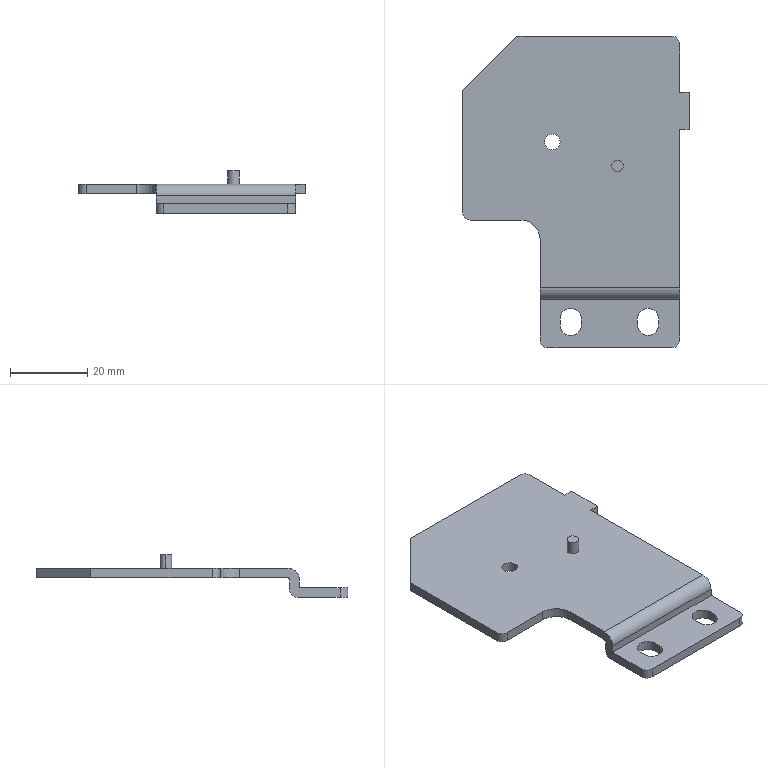Part | NX | features BREP 1 | 1 solid | 38 faces | box 58.5 x 80.5 x 11 mm | volume 9624 mm3 | plane 22 | cylinder 16 | commonest cylinder face diameters 4 x7 5.5 x4 3 x2 1 x1 6 x1 10 x1
STEP:
#1=CARTESIAN_POINT('',(-2.875,12.95,-2.5));
#2=VERTEX_POINT('',#1);
#3=CARTESIAN_POINT('',(-6.875,12.95,-2.5));
#4=VERTEX_POINT('',#3);
#5=CARTESIAN_POINT('',(-4.875,12.95,-2.5));
#6=DIRECTION('',(0.,0.,-1.));
#7=DIRECTION('',(1.,0.,0.));
#8=AXIS2_PLACEMENT_3D('',#5,#6,#7);
#9=CIRCLE('',#8,2.);
#10=EDGE_CURVE('',#2,#4,#9,.T.);
#11=ORIENTED_EDGE('',*,*,#10,.T.);
#12=CARTESIAN_POINT('',(-6.875,12.95,0.));
#13=VERTEX_POINT('',#12);
#14=CARTESIAN_POINT('',(-6.875,12.95,-1.));
#15=DIRECTION('',(0.,0.,1.));
#16=VECTOR('',#15,1000.);
#17=LINE('',#14,#16);
#18=EDGE_CURVE('',#4,#13,#17,.T.);
#19=ORIENTED_EDGE('',*,*,#18,.T.);
#20=CARTESIAN_POINT('',(-2.875,12.95,0.));
#21=VERTEX_POINT('',#20);
#22=CARTESIAN_POINT('',(-4.875,12.95,0.));
#23=DIRECTION('',(0.,0.,-1.));
#24=DIRECTION('',(1.,0.,0.));
#25=AXIS2_PLACEMENT_3D('',#22,#23,#24);
#26=CIRCLE('',#25,2.);
#27=EDGE_CURVE('',#21,#13,#26,.T.);
#28=ORIENTED_EDGE('',*,*,#27,.F.);
#29=CARTESIAN_POINT('',(-2.875,12.95,-1.));
#30=DIRECTION('',(0.,0.,1.));
#31=VECTOR('',#30,1000.);
#32=LINE('',#29,#31);
#33=EDGE_CURVE('',#2,#21,#32,.T.);
#34=ORIENTED_EDGE('',*,*,#33,.F.);
#35=EDGE_LOOP('',(#11,#19,#28,#34));
#36=FACE_BOUND('',#35,.T.);
#37=CARTESIAN_POINT('',(-4.875,12.95,-1.));
#38=DIRECTION('',(0.,0.,1.));
#39=DIRECTION('',(-1.,0.,0.));
#40=AXIS2_PLACEMENT_3D('',#37,#38,#39);
#41=CYLINDRICAL_SURFACE('',#40,2.);
#42=ADVANCED_FACE('',(#36),#41,.F.);
#43=CARTESIAN_POINT('',(10.5,6.75,3.5));
#44=VERTEX_POINT('',#43);
#45=CARTESIAN_POINT('',(13.5,6.75,3.5));
#46=VERTEX_POINT('',#45);
#47=CARTESIAN_POINT('',(12.,6.75,3.5));
#48=DIRECTION('',(0.,0.,-1.));
#49=DIRECTION('',(-1.,0.,0.));
#50=AXIS2_PLACEMENT_3D('',#47,#48,#49);
#51=CIRCLE('',#50,1.5);
#52=EDGE_CURVE('',#44,#46,#51,.T.);
#53=ORIENTED_EDGE('',*,*,#52,.T.);
#54=CARTESIAN_POINT('',(13.5,6.75,0.));
#55=VERTEX_POINT('',#54);
#56=CARTESIAN_POINT('',(13.5,6.75,-2.5));
#57=DIRECTION('',(0.,0.,-1.));
#58=VECTOR('',#57,1000.);
#59=LINE('',#56,#58);
#60=EDGE_CURVE('',#55,#46,#59,.F.);
#61=ORIENTED_EDGE('',*,*,#60,.F.);
#62=CARTESIAN_POINT('',(10.5,6.75,0.));
#63=VERTEX_POINT('',#62);
#64=CARTESIAN_POINT('',(12.,6.75,0.));
#65=DIRECTION('',(0.,0.,-1.));
#66=DIRECTION('',(-1.,0.,0.));
#67=AXIS2_PLACEMENT_3D('',#64,#65,#66);
#68=CIRCLE('',#67,1.5);
#69=EDGE_CURVE('',#63,#55,#68,.T.);
#70=ORIENTED_EDGE('',*,*,#69,.F.);
#71=CARTESIAN_POINT('',(10.5,6.75,-2.5));
#72=DIRECTION('',(0.,0.,-1.));
#73=VECTOR('',#72,1000.);
#74=LINE('',#71,#73);
#75=EDGE_CURVE('',#63,#44,#74,.F.);
#76=ORIENTED_EDGE('',*,*,#75,.T.);
#77=EDGE_LOOP('',(#53,#61,#70,#76));
#78=FACE_BOUND('',#77,.T.);
#79=CARTESIAN_POINT('',(12.,6.75,-2.5));
#80=DIRECTION('',(0.,0.,-1.));
#81=DIRECTION('',(1.,0.,0.));
#82=AXIS2_PLACEMENT_3D('',#79,#80,#81);
#83=CYLINDRICAL_SURFACE('',#82,1.5);
#84=ADVANCED_FACE('',(#78),#83,.T.);
#85=CARTESIAN_POINT('',(-14.,40.25,-2.5));
#86=VERTEX_POINT('',#85);
#87=CARTESIAN_POINT('',(-28.,26.25,-2.5));
#88=VERTEX_POINT('',#87);
#89=CARTESIAN_POINT('',(-14.,40.25,-2.5));
#90=DIRECTION('',(-0.7071,-0.7071,0.));
#91=VECTOR('',#90,1000.);
#92=LINE('',#89,#91);
#93=EDGE_CURVE('',#86,#88,#92,.T.);
#94=ORIENTED_EDGE('',*,*,#93,.F.);
#95=CARTESIAN_POINT('',(26.,40.25,-2.5));
#96=VERTEX_POINT('',#95);
#97=CARTESIAN_POINT('',(38.,40.25,-2.5));
#98=DIRECTION('',(-1.,0.,0.));
#99=VECTOR('',#98,1000.);
#100=LINE('',#97,#99);
#101=EDGE_CURVE('',#96,#86,#100,.T.);
#102=ORIENTED_EDGE('',*,*,#101,.F.);
#103=CARTESIAN_POINT('',(28.,38.25,-2.5));
#104=VERTEX_POINT('',#103);
#105=CARTESIAN_POINT('',(26.,38.25,-2.5));
#106=DIRECTION('',(0.,0.,1.));
#107=DIRECTION('',(1.,0.,0.));
#108=AXIS2_PLACEMENT_3D('',#105,#106,#107);
#109=CIRCLE('',#108,2.);
#110=EDGE_CURVE('',#104,#96,#109,.T.);
#111=ORIENTED_EDGE('',*,*,#110,.F.);
#112=CARTESIAN_POINT('',(28.,25.75,-2.5));
#113=VERTEX_POINT('',#112);
#114=CARTESIAN_POINT('',(28.,-7.834,-2.5));
#115=DIRECTION('',(0.,1.,0.));
#116=VECTOR('',#115,1000.);
#117=LINE('',#114,#116);
#118=EDGE_CURVE('',#113,#104,#117,.T.);
#119=ORIENTED_EDGE('',*,*,#118,.F.);
#120=CARTESIAN_POINT('',(30.5,25.75,-2.5));
#121=VERTEX_POINT('',#120);
#122=CARTESIAN_POINT('',(38.,25.75,-2.5));
#123=DIRECTION('',(-1.,0.,0.));
#124=VECTOR('',#123,1000.);
#125=LINE('',#122,#124);
#126=EDGE_CURVE('',#121,#113,#125,.T.);
#127=ORIENTED_EDGE('',*,*,#126,.F.);
#128=CARTESIAN_POINT('',(30.5,16.25,-2.5));
#129=VERTEX_POINT('',#128);
#130=CARTESIAN_POINT('',(30.5,-7.834,-2.5));
#131=DIRECTION('',(0.,1.,0.));
#132=VECTOR('',#131,1000.);
#133=LINE('',#130,#132);
#134=EDGE_CURVE('',#129,#121,#133,.T.);
#135=ORIENTED_EDGE('',*,*,#134,.F.);
#136=CARTESIAN_POINT('',(28.,16.25,-2.5));
#137=VERTEX_POINT('',#136);
#138=CARTESIAN_POINT('',(38.,16.25,-2.5));
#139=DIRECTION('',(1.,0.,0.));
#140=VECTOR('',#139,1000.);
#141=LINE('',#138,#140);
#142=EDGE_CURVE('',#137,#129,#141,.T.);
#143=ORIENTED_EDGE('',*,*,#142,.F.);
#144=CARTESIAN_POINT('',(28.,-24.768,-2.5));
#145=VERTEX_POINT('',#144);
#146=CARTESIAN_POINT('',(28.,-7.834,-2.5));
#147=DIRECTION('',(0.,1.,0.));
#148=VECTOR('',#147,1000.);
#149=LINE('',#146,#148);
#150=EDGE_CURVE('',#145,#137,#149,.T.);
#151=ORIENTED_EDGE('',*,*,#150,.F.);
#152=CARTESIAN_POINT('',(-8.,-24.768,-2.5));
#153=VERTEX_POINT('',#152);
#154=CARTESIAN_POINT('',(38.,-24.768,-2.5));
#155=DIRECTION('',(1.,0.,0.));
#156=VECTOR('',#155,1000.);
#157=LINE('',#154,#156);
#158=EDGE_CURVE('',#153,#145,#157,.T.);
#159=ORIENTED_EDGE('',*,*,#158,.F.);
#160=CARTESIAN_POINT('',(-8.,-12.25,-2.5));
#161=VERTEX_POINT('',#160);
#162=CARTESIAN_POINT('',(-8.,-7.834,-2.5));
#163=DIRECTION('',(0.,-1.,0.));
#164=VECTOR('',#163,1000.);
#165=LINE('',#162,#164);
#166=EDGE_CURVE('',#161,#153,#165,.T.);
#167=ORIENTED_EDGE('',*,*,#166,.F.);
#168=CARTESIAN_POINT('',(-13.,-7.25,-2.5));
#169=VERTEX_POINT('',#168);
#170=CARTESIAN_POINT('',(-13.,-12.25,-2.5));
#171=DIRECTION('',(0.,0.,-1.));
#172=DIRECTION('',(1.,0.,0.));
#173=AXIS2_PLACEMENT_3D('',#170,#171,#172);
#174=CIRCLE('',#173,5.);
#175=EDGE_CURVE('',#169,#161,#174,.T.);
#176=ORIENTED_EDGE('',*,*,#175,.F.);
#177=CARTESIAN_POINT('',(-26.,-7.25,-2.5));
#178=VERTEX_POINT('',#177);
#179=CARTESIAN_POINT('',(38.,-7.25,-2.5));
#180=DIRECTION('',(1.,0.,0.));
#181=VECTOR('',#180,1000.);
#182=LINE('',#179,#181);
#183=EDGE_CURVE('',#178,#169,#182,.T.);
#184=ORIENTED_EDGE('',*,*,#183,.F.);
#185=CARTESIAN_POINT('',(-28.,-5.25,-2.5));
#186=VERTEX_POINT('',#185);
#187=CARTESIAN_POINT('',(-26.,-5.25,-2.5));
#188=DIRECTION('',(0.,0.,1.));
#189=DIRECTION('',(1.,0.,0.));
#190=AXIS2_PLACEMENT_3D('',#187,#188,#189);
#191=CIRCLE('',#190,2.);
#192=EDGE_CURVE('',#186,#178,#191,.T.);
#193=ORIENTED_EDGE('',*,*,#192,.F.);
#194=CARTESIAN_POINT('',(-28.,-7.834,-2.5));
#195=DIRECTION('',(0.,-1.,0.));
#196=VECTOR('',#195,1000.);
#197=LINE('',#194,#196);
#198=EDGE_CURVE('',#88,#186,#197,.T.);
#199=ORIENTED_EDGE('',*,*,#198,.F.);
#200=EDGE_LOOP('',(#94,#102,#111,#119,#127,#135,#143,#151,#159,#167,#176,#184,#193,#199));
#201=FACE_BOUND('',#200,.T.);
#202=ORIENTED_EDGE('',*,*,#10,.F.);
#203=CARTESIAN_POINT('',(-4.875,12.95,-2.5));
#204=DIRECTION('',(0.,0.,-1.));
#205=DIRECTION('',(1.,0.,0.));
#206=AXIS2_PLACEMENT_3D('',#203,#204,#205);
#207=CIRCLE('',#206,2.);
#208=EDGE_CURVE('',#4,#2,#207,.T.);
#209=ORIENTED_EDGE('',*,*,#208,.F.);
#210=EDGE_LOOP('',(#202,#209));
#211=FACE_BOUND('',#210,.T.);
#212=CARTESIAN_POINT('',(38.,-7.834,-2.5));
#213=DIRECTION('',(0.,0.,1.));
#214=DIRECTION('',(-1.,0.,0.));
#215=AXIS2_PLACEMENT_3D('',#212,#213,#214);
#216=PLANE('',#215);
#217=ADVANCED_FACE('',(#201,#211),#216,.F.);
#218=ORIENTED_EDGE('',*,*,#198,.T.);
#219=CARTESIAN_POINT('',(-28.,-5.25,0.));
#220=VERTEX_POINT('',#219);
#221=CARTESIAN_POINT('',(-28.,-5.25,-1.));
#222=DIRECTION('',(0.,0.,-1.));
#223=VECTOR('',#222,1000.);
#224=LINE('',#221,#223);
#225=EDGE_CURVE('',#220,#186,#224,.T.);
#226=ORIENTED_EDGE('',*,*,#225,.F.);
#227=CARTESIAN_POINT('',(-28.,26.25,0.));
#228=VERTEX_POINT('',#227);
#229=CARTESIAN_POINT('',(-28.,-7.834,0.));
#230=DIRECTION('',(0.,-1.,0.));
#231=VECTOR('',#230,1000.);
#232=LINE('',#229,#231);
#233=EDGE_CURVE('',#228,#220,#232,.T.);
#234=ORIENTED_EDGE('',*,*,#233,.F.);
#235=CARTESIAN_POINT('',(-28.,26.25,-1.));
#236=DIRECTION('',(0.,0.,1.));
#237=VECTOR('',#236,1000.);
#238=LINE('',#235,#237);
#239=EDGE_CURVE('',#88,#228,#238,.T.);
#240=ORIENTED_EDGE('',*,*,#239,.F.);
#241=EDGE_LOOP('',(#218,#226,#234,#240));
#242=FACE_BOUND('',#241,.T.);
#243=CARTESIAN_POINT('',(-28.,-7.834,-1.));
#244=DIRECTION('',(1.,0.,0.));
#245=DIRECTION('',(0.,0.,1.));
#246=AXIS2_PLACEMENT_3D('',#243,#244,#245);
#247=PLANE('',#246);
#248=ADVANCED_FACE('',(#242),#247,.F.);
#249=ORIENTED_EDGE('',*,*,#239,.T.);
#250=CARTESIAN_POINT('',(-14.,40.25,0.));
#251=VERTEX_POINT('',#250);
#252=CARTESIAN_POINT('',(-14.,40.25,0.));
#253=DIRECTION('',(0.7071,0.7071,0.));
#254=VECTOR('',#253,1000.);
#255=LINE('',#252,#254);
#256=EDGE_CURVE('',#228,#251,#255,.T.);
#257=ORIENTED_EDGE('',*,*,#256,.T.);
#258=CARTESIAN_POINT('',(-14.,40.25,-1.));
#259=DIRECTION('',(0.,0.,-1.));
#260=VECTOR('',#259,1000.);
#261=LINE('',#258,#260);
#262=EDGE_CURVE('',#251,#86,#261,.T.);
#263=ORIENTED_EDGE('',*,*,#262,.T.);
#264=ORIENTED_EDGE('',*,*,#93,.T.);
#265=EDGE_LOOP('',(#249,#257,#263,#264));
#266=FACE_BOUND('',#265,.T.);
#267=CARTESIAN_POINT('',(-14.,40.25,-1.));
#268=DIRECTION('',(-0.7071,0.7071,0.));
#269=DIRECTION('',(0.7071,0.7071,0.));
#270=AXIS2_PLACEMENT_3D('',#267,#268,#269);
#271=PLANE('',#270);
#272=ADVANCED_FACE('',(#266),#271,.T.);
#273=ORIENTED_EDGE('',*,*,#101,.T.);
#274=ORIENTED_EDGE('',*,*,#262,.F.);
#275=CARTESIAN_POINT('',(26.,40.25,0.));
#276=VERTEX_POINT('',#275);
#277=CARTESIAN_POINT('',(38.,40.25,0.));
#278=DIRECTION('',(-1.,0.,0.));
#279=VECTOR('',#278,1000.);
#280=LINE('',#277,#279);
#281=EDGE_CURVE('',#276,#251,#280,.T.);
#282=ORIENTED_EDGE('',*,*,#281,.F.);
#283=CARTESIAN_POINT('',(26.,40.25,-1.));
#284=DIRECTION('',(0.,0.,1.));
#285=VECTOR('',#284,1000.);
#286=LINE('',#283,#285);
#287=EDGE_CURVE('',#96,#276,#286,.T.);
#288=ORIENTED_EDGE('',*,*,#287,.F.);
#289=EDGE_LOOP('',(#273,#274,#282,#288));
#290=FACE_BOUND('',#289,.T.);
#291=CARTESIAN_POINT('',(38.,40.25,-1.));
#292=DIRECTION('',(0.,-1.,0.));
#293=DIRECTION('',(0.,0.,1.));
#294=AXIS2_PLACEMENT_3D('',#291,#292,#293);
#295=PLANE('',#294);
#296=ADVANCED_FACE('',(#290),#295,.F.);
#297=ORIENTED_EDGE('',*,*,#287,.T.);
#298=CARTESIAN_POINT('',(28.,38.25,0.));
#299=VERTEX_POINT('',#298);
#300=CARTESIAN_POINT('',(26.,38.25,0.));
#301=DIRECTION('',(0.,0.,-1.));
#302=DIRECTION('',(1.,0.,0.));
#303=AXIS2_PLACEMENT_3D('',#300,#301,#302);
#304=CIRCLE('',#303,2.);
#305=EDGE_CURVE('',#276,#299,#304,.T.);
#306=ORIENTED_EDGE('',*,*,#305,.T.);
#307=CARTESIAN_POINT('',(28.,38.25,-1.));
#308=DIRECTION('',(0.,0.,-1.));
#309=VECTOR('',#308,1000.);
#310=LINE('',#307,#309);
#311=EDGE_CURVE('',#299,#104,#310,.T.);
#312=ORIENTED_EDGE('',*,*,#311,.T.);
#313=ORIENTED_EDGE('',*,*,#110,.T.);
#314=EDGE_LOOP('',(#297,#306,#312,#313));
#315=FACE_BOUND('',#314,.T.);
#316=CARTESIAN_POINT('',(26.,38.25,-1.));
#317=DIRECTION('',(0.,0.,1.));
#318=DIRECTION('',(-1.,0.,0.));
#319=AXIS2_PLACEMENT_3D('',#316,#317,#318);
#320=CYLINDRICAL_SURFACE('',#319,2.);
#321=ADVANCED_FACE('',(#315),#320,.T.);
#322=ORIENTED_EDGE('',*,*,#118,.T.);
#323=ORIENTED_EDGE('',*,*,#311,.F.);
#324=CARTESIAN_POINT('',(28.,25.75,0.));
#325=VERTEX_POINT('',#324);
#326=CARTESIAN_POINT('',(28.,-36.323,0.));
#327=DIRECTION('',(0.,1.,0.));
#328=VECTOR('',#327,1000.);
#329=LINE('',#326,#328);
#330=EDGE_CURVE('',#325,#299,#329,.T.);
#331=ORIENTED_EDGE('',*,*,#330,.F.);
#332=CARTESIAN_POINT('',(28.,25.75,-6.));
#333=DIRECTION('',(0.,0.,1.));
#334=VECTOR('',#333,1000.);
#335=LINE('',#332,#334);
#336=EDGE_CURVE('',#113,#325,#335,.T.);
#337=ORIENTED_EDGE('',*,*,#336,.F.);
#338=EDGE_LOOP('',(#322,#323,#331,#337));
#339=FACE_BOUND('',#338,.T.);
#340=CARTESIAN_POINT('',(28.,-36.323,-6.));
#341=DIRECTION('',(-1.,0.,0.));
#342=DIRECTION('',(0.,0.,-1.));
#343=AXIS2_PLACEMENT_3D('',#340,#341,#342);
#344=PLANE('',#343);
#345=ADVANCED_FACE('',(#339),#344,.F.);
#346=CARTESIAN_POINT('',(30.5,25.75,0.));
#347=VERTEX_POINT('',#346);
#348=CARTESIAN_POINT('',(30.5,25.75,-1.));
#349=DIRECTION('',(0.,0.,1.));
#350=VECTOR('',#349,1000.);
#351=LINE('',#348,#350);
#352=EDGE_CURVE('',#121,#347,#351,.T.);
#353=ORIENTED_EDGE('',*,*,#352,.F.);
#354=ORIENTED_EDGE('',*,*,#126,.T.);
#355=ORIENTED_EDGE('',*,*,#336,.T.);
#356=CARTESIAN_POINT('',(28.,25.75,0.));
#357=DIRECTION('',(-1.,0.,0.));
#358=VECTOR('',#357,1000.);
#359=LINE('',#356,#358);
#360=EDGE_CURVE('',#347,#325,#359,.T.);
#361=ORIENTED_EDGE('',*,*,#360,.F.);
#362=EDGE_LOOP('',(#353,#354,#355,#361));
#363=FACE_BOUND('',#362,.T.);
#364=CARTESIAN_POINT('',(28.,25.75,-1.));
#365=DIRECTION('',(0.,-1.,0.));
#366=DIRECTION('',(0.,0.,1.));
#367=AXIS2_PLACEMENT_3D('',#364,#365,#366);
#368=PLANE('',#367);
#369=ADVANCED_FACE('',(#363),#368,.F.);
#370=ORIENTED_EDGE('',*,*,#134,.T.);
#371=ORIENTED_EDGE('',*,*,#352,.T.);
#372=CARTESIAN_POINT('',(30.5,16.25,0.));
#373=VERTEX_POINT('',#372);
#374=CARTESIAN_POINT('',(30.5,16.25,0.));
#375=DIRECTION('',(0.,1.,0.));
#376=VECTOR('',#375,1000.);
#377=LINE('',#374,#376);
#378=EDGE_CURVE('',#373,#347,#377,.T.);
#379=ORIENTED_EDGE('',*,*,#378,.F.);
#380=CARTESIAN_POINT('',(30.5,16.25,-1.));
#381=DIRECTION('',(0.,0.,1.));
#382=VECTOR('',#381,1000.);
#383=LINE('',#380,#382);
#384=EDGE_CURVE('',#129,#373,#383,.T.);
#385=ORIENTED_EDGE('',*,*,#384,.F.);
#386=EDGE_LOOP('',(#370,#371,#379,#385));
#387=FACE_BOUND('',#386,.T.);
#388=CARTESIAN_POINT('',(30.5,16.25,-1.));
#389=DIRECTION('',(-1.,0.,0.));
#390=DIRECTION('',(0.,0.,-1.));
#391=AXIS2_PLACEMENT_3D('',#388,#389,#390);
#392=PLANE('',#391);
#393=ADVANCED_FACE('',(#387),#392,.F.);
#394=CARTESIAN_POINT('',(28.,16.25,0.));
#395=VERTEX_POINT('',#394);
#396=CARTESIAN_POINT('',(28.,16.25,-1.));
#397=DIRECTION('',(0.,0.,1.));
#398=VECTOR('',#397,1000.);
#399=LINE('',#396,#398);
#400=EDGE_CURVE('',#137,#395,#399,.T.);
#401=ORIENTED_EDGE('',*,*,#400,.F.);
#402=ORIENTED_EDGE('',*,*,#142,.T.);
#403=ORIENTED_EDGE('',*,*,#384,.T.);
#404=CARTESIAN_POINT('',(28.,16.25,0.));
#405=DIRECTION('',(1.,0.,0.));
#406=VECTOR('',#405,1000.);
#407=LINE('',#404,#406);
#408=EDGE_CURVE('',#395,#373,#407,.T.);
#409=ORIENTED_EDGE('',*,*,#408,.F.);
#410=EDGE_LOOP('',(#401,#402,#403,#409));
#411=FACE_BOUND('',#410,.T.);
#412=CARTESIAN_POINT('',(28.,16.25,-1.));
#413=DIRECTION('',(0.,1.,0.));
#414=DIRECTION('',(0.,0.,-1.));
#415=AXIS2_PLACEMENT_3D('',#412,#413,#414);
#416=PLANE('',#415);
#417=ADVANCED_FACE('',(#411),#416,.F.);
#418=CARTESIAN_POINT('',(28.,-27.768,-3.));
#419=VERTEX_POINT('',#418);
#420=CARTESIAN_POINT('',(28.,-24.768,0.));
#421=VERTEX_POINT('',#420);
#422=CARTESIAN_POINT('',(28.,-24.768,-3.));
#423=DIRECTION('',(-1.,0.,0.));
#424=DIRECTION('',(0.,0.,1.));
#425=AXIS2_PLACEMENT_3D('',#422,#423,#424);
#426=CIRCLE('',#425,3.);
#427=EDGE_CURVE('',#419,#421,#426,.T.);
#428=ORIENTED_EDGE('',*,*,#427,.F.);
#429=CARTESIAN_POINT('',(28.,-27.768,-5.));
#430=VERTEX_POINT('',#429);
#431=CARTESIAN_POINT('',(28.,-27.768,-6.));
#432=DIRECTION('',(0.,0.,1.));
#433=VECTOR('',#432,1000.);
#434=LINE('',#431,#433);
#435=EDGE_CURVE('',#430,#419,#434,.T.);
#436=ORIENTED_EDGE('',*,*,#435,.F.);
#437=CARTESIAN_POINT('',(28.,-38.25,-5.));
#438=VERTEX_POINT('',#437);
#439=CARTESIAN_POINT('',(28.,-36.323,-5.));
#440=DIRECTION('',(0.,1.,0.));
#441=VECTOR('',#440,1000.);
#442=LINE('',#439,#441);
#443=EDGE_CURVE('',#438,#430,#442,.T.);
#444=ORIENTED_EDGE('',*,*,#443,.F.);
#445=CARTESIAN_POINT('',(28.,-38.25,-7.5));
#446=VERTEX_POINT('',#445);
#447=CARTESIAN_POINT('',(28.,-38.25,-6.));
#448=DIRECTION('',(0.,0.,1.));
#449=VECTOR('',#448,1000.);
#450=LINE('',#447,#449);
#451=EDGE_CURVE('',#446,#438,#450,.T.);
#452=ORIENTED_EDGE('',*,*,#451,.F.);
#453=CARTESIAN_POINT('',(28.,-27.268,-7.5));
#454=VERTEX_POINT('',#453);
#455=CARTESIAN_POINT('',(28.,-36.323,-7.5));
#456=DIRECTION('',(0.,-1.,0.));
#457=VECTOR('',#456,1000.);
#458=LINE('',#455,#457);
#459=EDGE_CURVE('',#454,#446,#458,.T.);
#460=ORIENTED_EDGE('',*,*,#459,.F.);
#461=CARTESIAN_POINT('',(28.,-25.268,-5.5));
#462=VERTEX_POINT('',#461);
#463=CARTESIAN_POINT('',(28.,-27.268,-5.5));
#464=DIRECTION('',(-1.,0.,0.));
#465=DIRECTION('',(0.,0.,1.));
#466=AXIS2_PLACEMENT_3D('',#463,#464,#465);
#467=CIRCLE('',#466,2.);
#468=EDGE_CURVE('',#462,#454,#467,.T.);
#469=ORIENTED_EDGE('',*,*,#468,.F.);
#470=CARTESIAN_POINT('',(28.,-25.268,-3.));
#471=VERTEX_POINT('',#470);
#472=CARTESIAN_POINT('',(28.,-25.268,-6.));
#473=DIRECTION('',(0.,0.,-1.));
#474=VECTOR('',#473,1000.);
#475=LINE('',#472,#474);
#476=EDGE_CURVE('',#471,#462,#475,.T.);
#477=ORIENTED_EDGE('',*,*,#476,.F.);
#478=CARTESIAN_POINT('',(28.,-24.768,-3.));
#479=DIRECTION('',(1.,0.,0.));
#480=DIRECTION('',(0.,0.,1.));
#481=AXIS2_PLACEMENT_3D('',#478,#479,#480);
#482=CIRCLE('',#481,0.5);
#483=EDGE_CURVE('',#145,#471,#482,.T.);
#484=ORIENTED_EDGE('',*,*,#483,.F.);
#485=ORIENTED_EDGE('',*,*,#150,.T.);
#486=ORIENTED_EDGE('',*,*,#400,.T.);
#487=CARTESIAN_POINT('',(28.,-36.323,0.));
#488=DIRECTION('',(0.,1.,0.));
#489=VECTOR('',#488,1000.);
#490=LINE('',#487,#489);
#491=EDGE_CURVE('',#421,#395,#490,.T.);
#492=ORIENTED_EDGE('',*,*,#491,.F.);
#493=EDGE_LOOP('',(#428,#436,#444,#452,#460,#469,#477,#484,#485,#486,#492));
#494=FACE_BOUND('',#493,.T.);
#495=CARTESIAN_POINT('',(28.,-36.323,-6.));
#496=DIRECTION('',(-1.,0.,0.));
#497=DIRECTION('',(0.,0.,-1.));
#498=AXIS2_PLACEMENT_3D('',#495,#496,#497);
#499=PLANE('',#498);
#500=ADVANCED_FACE('',(#494),#499,.F.);
#501=CARTESIAN_POINT('',(-8.,-25.268,-3.));
#502=VERTEX_POINT('',#501);
#503=CARTESIAN_POINT('',(-8.,-24.768,-3.));
#504=DIRECTION('',(1.,0.,0.));
#505=DIRECTION('',(0.,0.,1.));
#506=AXIS2_PLACEMENT_3D('',#503,#504,#505);
#507=CIRCLE('',#506,0.5);
#508=EDGE_CURVE('',#153,#502,#507,.T.);
#509=ORIENTED_EDGE('',*,*,#508,.F.);
#510=ORIENTED_EDGE('',*,*,#158,.T.);
#511=ORIENTED_EDGE('',*,*,#483,.T.);
#512=CARTESIAN_POINT('',(46.085,-25.268,-3.));
#513=DIRECTION('',(1.,0.,0.));
#514=VECTOR('',#513,1000.);
#515=LINE('',#512,#514);
#516=EDGE_CURVE('',#502,#471,#515,.T.);
#517=ORIENTED_EDGE('',*,*,#516,.F.);
#518=EDGE_LOOP('',(#509,#510,#511,#517));
#519=FACE_BOUND('',#518,.T.);
#520=CARTESIAN_POINT('',(46.085,-24.768,-3.));
#521=DIRECTION('',(-1.,0.,0.));
#522=DIRECTION('',(0.,0.,-1.));
#523=AXIS2_PLACEMENT_3D('',#520,#521,#522);
#524=CYLINDRICAL_SURFACE('',#523,0.5);
#525=ADVANCED_FACE('',(#519),#524,.F.);
#526=CARTESIAN_POINT('',(-8.,-27.768,-3.));
#527=VERTEX_POINT('',#526);
#528=CARTESIAN_POINT('',(-8.,-27.768,-5.));
#529=VERTEX_POINT('',#528);
#530=CARTESIAN_POINT('',(-8.,-27.768,-6.));
#531=DIRECTION('',(0.,0.,-1.));
#532=VECTOR('',#531,1000.);
#533=LINE('',#530,#532);
#534=EDGE_CURVE('',#527,#529,#533,.T.);
#535=ORIENTED_EDGE('',*,*,#534,.F.);
#536=CARTESIAN_POINT('',(-8.,-24.768,0.));
#537=VERTEX_POINT('',#536);
#538=CARTESIAN_POINT('',(-8.,-24.768,-3.));
#539=DIRECTION('',(1.,0.,0.));
#540=DIRECTION('',(0.,0.,1.));
#541=AXIS2_PLACEMENT_3D('',#538,#539,#540);
#542=CIRCLE('',#541,3.);
#543=EDGE_CURVE('',#537,#527,#542,.T.);
#544=ORIENTED_EDGE('',*,*,#543,.F.);
#545=CARTESIAN_POINT('',(-8.,-12.25,0.));
#546=VERTEX_POINT('',#545);
#547=CARTESIAN_POINT('',(-8.,32.708,0.));
#548=DIRECTION('',(0.,-1.,0.));
#549=VECTOR('',#548,1000.);
#550=LINE('',#547,#549);
#551=EDGE_CURVE('',#546,#537,#550,.T.);
#552=ORIENTED_EDGE('',*,*,#551,.F.);
#553=CARTESIAN_POINT('',(-8.,-12.25,-6.));
#554=DIRECTION('',(0.,0.,1.));
#555=VECTOR('',#554,1000.);
#556=LINE('',#553,#555);
#557=EDGE_CURVE('',#161,#546,#556,.T.);
#558=ORIENTED_EDGE('',*,*,#557,.F.);
#559=ORIENTED_EDGE('',*,*,#166,.T.);
#560=ORIENTED_EDGE('',*,*,#508,.T.);
#561=CARTESIAN_POINT('',(-8.,-25.268,-5.5));
#562=VERTEX_POINT('',#561);
#563=CARTESIAN_POINT('',(-8.,-25.268,-6.));
#564=DIRECTION('',(0.,0.,1.));
#565=VECTOR('',#564,1000.);
#566=LINE('',#563,#565);
#567=EDGE_CURVE('',#562,#502,#566,.T.);
#568=ORIENTED_EDGE('',*,*,#567,.F.);
#569=CARTESIAN_POINT('',(-8.,-27.268,-7.5));
#570=VERTEX_POINT('',#569);
#571=CARTESIAN_POINT('',(-8.,-27.268,-5.5));
#572=DIRECTION('',(1.,0.,0.));
#573=DIRECTION('',(0.,0.,1.));
#574=AXIS2_PLACEMENT_3D('',#571,#572,#573);
#575=CIRCLE('',#574,2.);
#576=EDGE_CURVE('',#570,#562,#575,.T.);
#577=ORIENTED_EDGE('',*,*,#576,.F.);
#578=CARTESIAN_POINT('',(-8.,-38.25,-7.5));
#579=VERTEX_POINT('',#578);
#580=CARTESIAN_POINT('',(-8.,32.708,-7.5));
#581=DIRECTION('',(0.,1.,0.));
#582=VECTOR('',#581,1000.);
#583=LINE('',#580,#582);
#584=EDGE_CURVE('',#579,#570,#583,.T.);
#585=ORIENTED_EDGE('',*,*,#584,.F.);
#586=CARTESIAN_POINT('',(-8.,-38.25,-5.));
#587=VERTEX_POINT('',#586);
#588=CARTESIAN_POINT('',(-8.,-38.25,-6.));
#589=DIRECTION('',(0.,0.,-1.));
#590=VECTOR('',#589,1000.);
#591=LINE('',#588,#590);
#592=EDGE_CURVE('',#587,#579,#591,.T.);
#593=ORIENTED_EDGE('',*,*,#592,.F.);
#594=CARTESIAN_POINT('',(-8.,32.708,-5.));
#595=DIRECTION('',(0.,-1.,0.));
#596=VECTOR('',#595,1000.);
#597=LINE('',#594,#596);
#598=EDGE_CURVE('',#529,#587,#597,.T.);
#599=ORIENTED_EDGE('',*,*,#598,.F.);
#600=EDGE_LOOP('',(#535,#544,#552,#558,#559,#560,#568,#577,#585,#593,#599));
#601=FACE_BOUND('',#600,.T.);
#602=CARTESIAN_POINT('',(-8.,32.708,-6.));
#603=DIRECTION('',(1.,0.,0.));
#604=DIRECTION('',(0.,0.,1.));
#605=AXIS2_PLACEMENT_3D('',#602,#603,#604);
#606=PLANE('',#605);
#607=ADVANCED_FACE('',(#601),#606,.F.);
#608=CARTESIAN_POINT('',(-13.,-7.25,0.));
#609=VERTEX_POINT('',#608);
#610=CARTESIAN_POINT('',(-13.,-12.25,0.));
#611=DIRECTION('',(0.,0.,-1.));
#612=DIRECTION('',(1.,0.,0.));
#613=AXIS2_PLACEMENT_3D('',#610,#611,#612);
#614=CIRCLE('',#613,5.);
#615=EDGE_CURVE('',#609,#546,#614,.T.);
#616=ORIENTED_EDGE('',*,*,#615,.F.);
#617=CARTESIAN_POINT('',(-13.,-7.25,-1.));
#618=DIRECTION('',(0.,0.,1.));
#619=VECTOR('',#618,1000.);
#620=LINE('',#617,#619);
#621=EDGE_CURVE('',#169,#609,#620,.T.);
#622=ORIENTED_EDGE('',*,*,#621,.F.);
#623=ORIENTED_EDGE('',*,*,#175,.T.);
#624=ORIENTED_EDGE('',*,*,#557,.T.);
#625=EDGE_LOOP('',(#616,#622,#623,#624));
#626=FACE_BOUND('',#625,.T.);
#627=CARTESIAN_POINT('',(-13.,-12.25,-1.));
#628=DIRECTION('',(0.,0.,1.));
#629=DIRECTION('',(-1.,0.,0.));
#630=AXIS2_PLACEMENT_3D('',#627,#628,#629);
#631=CYLINDRICAL_SURFACE('',#630,5.);
#632=ADVANCED_FACE('',(#626),#631,.F.);
#633=ORIENTED_EDGE('',*,*,#621,.T.);
#634=CARTESIAN_POINT('',(-26.,-7.25,0.));
#635=VERTEX_POINT('',#634);
#636=CARTESIAN_POINT('',(38.,-7.25,0.));
#637=DIRECTION('',(-1.,0.,0.));
#638=VECTOR('',#637,1000.);
#639=LINE('',#636,#638);
#640=EDGE_CURVE('',#609,#635,#639,.T.);
#641=ORIENTED_EDGE('',*,*,#640,.T.);
#642=CARTESIAN_POINT('',(-26.,-7.25,-1.));
#643=DIRECTION('',(0.,0.,-1.));
#644=VECTOR('',#643,1000.);
#645=LINE('',#642,#644);
#646=EDGE_CURVE('',#635,#178,#645,.T.);
#647=ORIENTED_EDGE('',*,*,#646,.T.);
#648=ORIENTED_EDGE('',*,*,#183,.T.);
#649=EDGE_LOOP('',(#633,#641,#647,#648));
#650=FACE_BOUND('',#649,.T.);
#651=CARTESIAN_POINT('',(38.,-7.25,-1.));
#652=DIRECTION('',(0.,-1.,0.));
#653=DIRECTION('',(0.,0.,1.));
#654=AXIS2_PLACEMENT_3D('',#651,#652,#653);
#655=PLANE('',#654);
#656=ADVANCED_FACE('',(#650),#655,.T.);
#657=ORIENTED_EDGE('',*,*,#646,.F.);
#658=CARTESIAN_POINT('',(-26.,-5.25,0.));
#659=DIRECTION('',(0.,0.,-1.));
#660=DIRECTION('',(1.,0.,0.));
#661=AXIS2_PLACEMENT_3D('',#658,#659,#660);
#662=CIRCLE('',#661,2.);
#663=EDGE_CURVE('',#635,#220,#662,.T.);
#664=ORIENTED_EDGE('',*,*,#663,.T.);
#665=ORIENTED_EDGE('',*,*,#225,.T.);
#666=ORIENTED_EDGE('',*,*,#192,.T.);
#667=EDGE_LOOP('',(#657,#664,#665,#666));
#668=FACE_BOUND('',#667,.T.);
#669=CARTESIAN_POINT('',(-26.,-5.25,-1.));
#670=DIRECTION('',(0.,0.,1.));
#671=DIRECTION('',(-1.,0.,0.));
#672=AXIS2_PLACEMENT_3D('',#669,#670,#671);
#673=CYLINDRICAL_SURFACE('',#672,2.);
#674=ADVANCED_FACE('',(#668),#673,.T.);
#675=ORIENTED_EDGE('',*,*,#18,.F.);
#676=ORIENTED_EDGE('',*,*,#208,.T.);
#677=ORIENTED_EDGE('',*,*,#33,.T.);
#678=CARTESIAN_POINT('',(-4.875,12.95,0.));
#679=DIRECTION('',(0.,0.,-1.));
#680=DIRECTION('',(1.,0.,0.));
#681=AXIS2_PLACEMENT_3D('',#678,#679,#680);
#682=CIRCLE('',#681,2.);
#683=EDGE_CURVE('',#13,#21,#682,.T.);
#684=ORIENTED_EDGE('',*,*,#683,.F.);
#685=EDGE_LOOP('',(#675,#676,#677,#684));
#686=FACE_BOUND('',#685,.T.);
#687=CARTESIAN_POINT('',(-4.875,12.95,-1.));
#688=DIRECTION('',(0.,0.,1.));
#689=DIRECTION('',(-1.,0.,0.));
#690=AXIS2_PLACEMENT_3D('',#687,#688,#689);
#691=CYLINDRICAL_SURFACE('',#690,2.);
#692=ADVANCED_FACE('',(#686),#691,.F.);
#693=ORIENTED_EDGE('',*,*,#360,.T.);
#694=ORIENTED_EDGE('',*,*,#330,.T.);
#695=ORIENTED_EDGE('',*,*,#305,.F.);
#696=ORIENTED_EDGE('',*,*,#281,.T.);
#697=ORIENTED_EDGE('',*,*,#256,.F.);
#698=ORIENTED_EDGE('',*,*,#233,.T.);
#699=ORIENTED_EDGE('',*,*,#663,.F.);
#700=ORIENTED_EDGE('',*,*,#640,.F.);
#701=ORIENTED_EDGE('',*,*,#615,.T.);
#702=ORIENTED_EDGE('',*,*,#551,.T.);
#703=CARTESIAN_POINT('',(38.,-24.768,0.));
#704=DIRECTION('',(1.,0.,0.));
#705=VECTOR('',#704,1000.);
#706=LINE('',#703,#705);
#707=EDGE_CURVE('',#537,#421,#706,.T.);
#708=ORIENTED_EDGE('',*,*,#707,.T.);
#709=ORIENTED_EDGE('',*,*,#491,.T.);
#710=ORIENTED_EDGE('',*,*,#408,.T.);
#711=ORIENTED_EDGE('',*,*,#378,.T.);
#712=EDGE_LOOP('',(#693,#694,#695,#696,#697,#698,#699,#700,#701,#702,#708,#709,#710,#711));
#713=FACE_BOUND('',#712,.T.);
#714=ORIENTED_EDGE('',*,*,#27,.T.);
#715=ORIENTED_EDGE('',*,*,#683,.T.);
#716=EDGE_LOOP('',(#714,#715));
#717=FACE_BOUND('',#716,.T.);
#718=ORIENTED_EDGE('',*,*,#69,.T.);
#719=CARTESIAN_POINT('',(12.,6.75,0.));
#720=DIRECTION('',(0.,0.,-1.));
#721=DIRECTION('',(-1.,0.,0.));
#722=AXIS2_PLACEMENT_3D('',#719,#720,#721);
#723=CIRCLE('',#722,1.5);
#724=EDGE_CURVE('',#55,#63,#723,.T.);
#725=ORIENTED_EDGE('',*,*,#724,.T.);
#726=EDGE_LOOP('',(#718,#725));
#727=FACE_BOUND('',#726,.T.);
#728=CARTESIAN_POINT('',(38.,-7.834,0.));
#729=DIRECTION('',(0.,0.,1.));
#730=DIRECTION('',(-1.,0.,0.));
#731=AXIS2_PLACEMENT_3D('',#728,#729,#730);
#732=PLANE('',#731);
#733=ADVANCED_FACE('',(#713,#717,#727),#732,.T.);
#734=ORIENTED_EDGE('',*,*,#707,.F.);
#735=ORIENTED_EDGE('',*,*,#543,.T.);
#736=CARTESIAN_POINT('',(46.085,-27.768,-3.));
#737=DIRECTION('',(1.,0.,0.));
#738=VECTOR('',#737,1000.);
#739=LINE('',#736,#738);
#740=EDGE_CURVE('',#527,#419,#739,.T.);
#741=ORIENTED_EDGE('',*,*,#740,.T.);
#742=ORIENTED_EDGE('',*,*,#427,.T.);
#743=EDGE_LOOP('',(#734,#735,#741,#742));
#744=FACE_BOUND('',#743,.T.);
#745=CARTESIAN_POINT('',(46.085,-24.768,-3.));
#746=DIRECTION('',(-1.,0.,0.));
#747=DIRECTION('',(0.,0.,-1.));
#748=AXIS2_PLACEMENT_3D('',#745,#746,#747);
#749=CYLINDRICAL_SURFACE('',#748,3.);
#750=ADVANCED_FACE('',(#744),#749,.T.);
#751=ORIENTED_EDGE('',*,*,#740,.F.);
#752=ORIENTED_EDGE('',*,*,#534,.T.);
#753=CARTESIAN_POINT('',(38.,-27.768,-5.));
#754=DIRECTION('',(1.,0.,0.));
#755=VECTOR('',#754,1000.);
#756=LINE('',#753,#755);
#757=EDGE_CURVE('',#529,#430,#756,.T.);
#758=ORIENTED_EDGE('',*,*,#757,.T.);
#759=ORIENTED_EDGE('',*,*,#435,.T.);
#760=EDGE_LOOP('',(#751,#752,#758,#759));
#761=FACE_BOUND('',#760,.T.);
#762=CARTESIAN_POINT('',(38.,-27.768,15.898));
#763=DIRECTION('',(0.,-1.,0.));
#764=DIRECTION('',(0.,0.,1.));
#765=AXIS2_PLACEMENT_3D('',#762,#763,#764);
#766=PLANE('',#765);
#767=ADVANCED_FACE('',(#761),#766,.T.);
#768=ORIENTED_EDGE('',*,*,#757,.F.);
#769=ORIENTED_EDGE('',*,*,#598,.T.);
#770=CARTESIAN_POINT('',(-6.,-40.25,-5.));
#771=VERTEX_POINT('',#770);
#772=CARTESIAN_POINT('',(-6.,-38.25,-5.));
#773=DIRECTION('',(0.,0.,1.));
#774=DIRECTION('',(1.,0.,0.));
#775=AXIS2_PLACEMENT_3D('',#772,#773,#774);
#776=CIRCLE('',#775,2.);
#777=EDGE_CURVE('',#587,#771,#776,.T.);
#778=ORIENTED_EDGE('',*,*,#777,.T.);
#779=CARTESIAN_POINT('',(26.,-40.25,-5.));
#780=VERTEX_POINT('',#779);
#781=CARTESIAN_POINT('',(38.,-40.25,-5.));
#782=DIRECTION('',(1.,0.,0.));
#783=VECTOR('',#782,1000.);
#784=LINE('',#781,#783);
#785=EDGE_CURVE('',#771,#780,#784,.T.);
#786=ORIENTED_EDGE('',*,*,#785,.T.);
#787=CARTESIAN_POINT('',(26.,-38.25,-5.));
#788=DIRECTION('',(0.,0.,1.));
#789=DIRECTION('',(1.,0.,0.));
#790=AXIS2_PLACEMENT_3D('',#787,#788,#789);
#791=CIRCLE('',#790,2.);
#792=EDGE_CURVE('',#780,#438,#791,.T.);
#793=ORIENTED_EDGE('',*,*,#792,.T.);
#794=ORIENTED_EDGE('',*,*,#443,.T.);
#795=EDGE_LOOP('',(#768,#769,#778,#786,#793,#794));
#796=FACE_BOUND('',#795,.T.);
#797=CARTESIAN_POINT('',(17.125,-32.8,-5.));
#798=VERTEX_POINT('',#797);
#799=CARTESIAN_POINT('',(17.125,-34.3,-5.));
#800=VERTEX_POINT('',#799);
#801=CARTESIAN_POINT('',(17.125,-34.3,-5.));
#802=DIRECTION('',(0.,-1.,0.));
#803=VECTOR('',#802,1000.);
#804=LINE('',#801,#803);
#805=EDGE_CURVE('',#798,#800,#804,.T.);
#806=ORIENTED_EDGE('',*,*,#805,.F.);
#807=CARTESIAN_POINT('',(22.625,-32.8,-5.));
#808=VERTEX_POINT('',#807);
#809=CARTESIAN_POINT('',(19.875,-32.8,-5.));
#810=DIRECTION('',(0.,0.,-1.));
#811=DIRECTION('',(1.,0.,0.));
#812=AXIS2_PLACEMENT_3D('',#809,#810,#811);
#813=CIRCLE('',#812,2.75);
#814=EDGE_CURVE('',#798,#808,#813,.T.);
#815=ORIENTED_EDGE('',*,*,#814,.T.);
#816=CARTESIAN_POINT('',(22.625,-34.3,-5.));
#817=VERTEX_POINT('',#816);
#818=CARTESIAN_POINT('',(22.625,-34.3,-5.));
#819=DIRECTION('',(0.,1.,0.));
#820=VECTOR('',#819,1000.);
#821=LINE('',#818,#820);
#822=EDGE_CURVE('',#817,#808,#821,.T.);
#823=ORIENTED_EDGE('',*,*,#822,.F.);
#824=CARTESIAN_POINT('',(19.875,-34.3,-5.));
#825=DIRECTION('',(0.,0.,-1.));
#826=DIRECTION('',(1.,0.,0.));
#827=AXIS2_PLACEMENT_3D('',#824,#825,#826);
#828=CIRCLE('',#827,2.75);
#829=EDGE_CURVE('',#817,#800,#828,.T.);
#830=ORIENTED_EDGE('',*,*,#829,.T.);
#831=EDGE_LOOP('',(#806,#815,#823,#830));
#832=FACE_BOUND('',#831,.T.);
#833=CARTESIAN_POINT('',(-2.875,-32.8,-5.));
#834=VERTEX_POINT('',#833);
#835=CARTESIAN_POINT('',(-2.875,-34.3,-5.));
#836=VERTEX_POINT('',#835);
#837=CARTESIAN_POINT('',(-2.875,-34.3,-5.));
#838=DIRECTION('',(0.,-1.,0.));
#839=VECTOR('',#838,1000.);
#840=LINE('',#837,#839);
#841=EDGE_CURVE('',#834,#836,#840,.T.);
#842=ORIENTED_EDGE('',*,*,#841,.F.);
#843=CARTESIAN_POINT('',(2.625,-32.8,-5.));
#844=VERTEX_POINT('',#843);
#845=CARTESIAN_POINT('',(-0.125,-32.8,-5.));
#846=DIRECTION('',(0.,0.,-1.));
#847=DIRECTION('',(1.,0.,0.));
#848=AXIS2_PLACEMENT_3D('',#845,#846,#847);
#849=CIRCLE('',#848,2.75);
#850=EDGE_CURVE('',#834,#844,#849,.T.);
#851=ORIENTED_EDGE('',*,*,#850,.T.);
#852=CARTESIAN_POINT('',(2.625,-34.3,-5.));
#853=VERTEX_POINT('',#852);
#854=CARTESIAN_POINT('',(2.625,-34.3,-5.));
#855=DIRECTION('',(0.,1.,0.));
#856=VECTOR('',#855,1000.);
#857=LINE('',#854,#856);
#858=EDGE_CURVE('',#853,#844,#857,.T.);
#859=ORIENTED_EDGE('',*,*,#858,.F.);
#860=CARTESIAN_POINT('',(-0.125,-34.3,-5.));
#861=DIRECTION('',(0.,0.,-1.));
#862=DIRECTION('',(1.,0.,0.));
#863=AXIS2_PLACEMENT_3D('',#860,#861,#862);
#864=CIRCLE('',#863,2.75);
#865=EDGE_CURVE('',#853,#836,#864,.T.);
#866=ORIENTED_EDGE('',*,*,#865,.T.);
#867=EDGE_LOOP('',(#842,#851,#859,#866));
#868=FACE_BOUND('',#867,.T.);
#869=CARTESIAN_POINT('',(38.,-3.907,-5.));
#870=DIRECTION('',(0.,0.,1.));
#871=DIRECTION('',(-1.,0.,0.));
#872=AXIS2_PLACEMENT_3D('',#869,#870,#871);
#873=PLANE('',#872);
#874=ADVANCED_FACE('',(#796,#832,#868),#873,.T.);
#875=ORIENTED_EDGE('',*,*,#451,.T.);
#876=ORIENTED_EDGE('',*,*,#792,.F.);
#877=CARTESIAN_POINT('',(26.,-40.25,-7.5));
#878=VERTEX_POINT('',#877);
#879=CARTESIAN_POINT('',(26.,-40.25,-6.));
#880=DIRECTION('',(0.,0.,-1.));
#881=VECTOR('',#880,1000.);
#882=LINE('',#879,#881);
#883=EDGE_CURVE('',#780,#878,#882,.T.);
#884=ORIENTED_EDGE('',*,*,#883,.T.);
#885=CARTESIAN_POINT('',(26.,-38.25,-7.5));
#886=DIRECTION('',(0.,0.,1.));
#887=DIRECTION('',(1.,0.,0.));
#888=AXIS2_PLACEMENT_3D('',#885,#886,#887);
#889=CIRCLE('',#888,2.);
#890=EDGE_CURVE('',#878,#446,#889,.T.);
#891=ORIENTED_EDGE('',*,*,#890,.T.);
#892=EDGE_LOOP('',(#875,#876,#884,#891));
#893=FACE_BOUND('',#892,.T.);
#894=CARTESIAN_POINT('',(26.,-38.25,-6.));
#895=DIRECTION('',(0.,0.,1.));
#896=DIRECTION('',(-1.,0.,0.));
#897=AXIS2_PLACEMENT_3D('',#894,#895,#896);
#898=CYLINDRICAL_SURFACE('',#897,2.);
#899=ADVANCED_FACE('',(#893),#898,.T.);
#900=ORIENTED_EDGE('',*,*,#584,.T.);
#901=CARTESIAN_POINT('',(38.,-27.268,-7.5));
#902=DIRECTION('',(-1.,0.,0.));
#903=VECTOR('',#902,1000.);
#904=LINE('',#901,#903);
#905=EDGE_CURVE('',#454,#570,#904,.T.);
#906=ORIENTED_EDGE('',*,*,#905,.F.);
#907=ORIENTED_EDGE('',*,*,#459,.T.);
#908=ORIENTED_EDGE('',*,*,#890,.F.);
#909=CARTESIAN_POINT('',(-6.,-40.25,-7.5));
#910=VERTEX_POINT('',#909);
#911=CARTESIAN_POINT('',(38.,-40.25,-7.5));
#912=DIRECTION('',(1.,0.,0.));
#913=VECTOR('',#912,1000.);
#914=LINE('',#911,#913);
#915=EDGE_CURVE('',#910,#878,#914,.T.);
#916=ORIENTED_EDGE('',*,*,#915,.F.);
#917=CARTESIAN_POINT('',(-6.,-38.25,-7.5));
#918=DIRECTION('',(0.,0.,1.));
#919=DIRECTION('',(1.,0.,0.));
#920=AXIS2_PLACEMENT_3D('',#917,#918,#919);
#921=CIRCLE('',#920,2.);
#922=EDGE_CURVE('',#579,#910,#921,.T.);
#923=ORIENTED_EDGE('',*,*,#922,.F.);
#924=EDGE_LOOP('',(#900,#906,#907,#908,#916,#923));
#925=FACE_BOUND('',#924,.T.);
#926=CARTESIAN_POINT('',(17.125,-34.3,-7.5));
#927=VERTEX_POINT('',#926);
#928=CARTESIAN_POINT('',(17.125,-32.8,-7.5));
#929=VERTEX_POINT('',#928);
#930=CARTESIAN_POINT('',(17.125,-34.3,-7.5));
#931=DIRECTION('',(0.,1.,0.));
#932=VECTOR('',#931,1000.);
#933=LINE('',#930,#932);
#934=EDGE_CURVE('',#927,#929,#933,.T.);
#935=ORIENTED_EDGE('',*,*,#934,.F.);
#936=CARTESIAN_POINT('',(22.625,-34.3,-7.5));
#937=VERTEX_POINT('',#936);
#938=CARTESIAN_POINT('',(19.875,-34.3,-7.5));
#939=DIRECTION('',(0.,0.,-1.));
#940=DIRECTION('',(1.,0.,0.));
#941=AXIS2_PLACEMENT_3D('',#938,#939,#940);
#942=CIRCLE('',#941,2.75);
#943=EDGE_CURVE('',#937,#927,#942,.T.);
#944=ORIENTED_EDGE('',*,*,#943,.F.);
#945=CARTESIAN_POINT('',(22.625,-32.8,-7.5));
#946=VERTEX_POINT('',#945);
#947=CARTESIAN_POINT('',(22.625,-34.3,-7.5));
#948=DIRECTION('',(0.,-1.,0.));
#949=VECTOR('',#948,1000.);
#950=LINE('',#947,#949);
#951=EDGE_CURVE('',#946,#937,#950,.T.);
#952=ORIENTED_EDGE('',*,*,#951,.F.);
#953=CARTESIAN_POINT('',(19.875,-32.8,-7.5));
#954=DIRECTION('',(0.,0.,-1.));
#955=DIRECTION('',(1.,0.,0.));
#956=AXIS2_PLACEMENT_3D('',#953,#954,#955);
#957=CIRCLE('',#956,2.75);
#958=EDGE_CURVE('',#929,#946,#957,.T.);
#959=ORIENTED_EDGE('',*,*,#958,.F.);
#960=EDGE_LOOP('',(#935,#944,#952,#959));
#961=FACE_BOUND('',#960,.T.);
#962=CARTESIAN_POINT('',(-2.875,-34.3,-7.5));
#963=VERTEX_POINT('',#962);
#964=CARTESIAN_POINT('',(-2.875,-32.8,-7.5));
#965=VERTEX_POINT('',#964);
#966=CARTESIAN_POINT('',(-2.875,-34.3,-7.5));
#967=DIRECTION('',(0.,1.,0.));
#968=VECTOR('',#967,1000.);
#969=LINE('',#966,#968);
#970=EDGE_CURVE('',#963,#965,#969,.T.);
#971=ORIENTED_EDGE('',*,*,#970,.F.);
#972=CARTESIAN_POINT('',(2.625,-34.3,-7.5));
#973=VERTEX_POINT('',#972);
#974=CARTESIAN_POINT('',(-0.125,-34.3,-7.5));
#975=DIRECTION('',(0.,0.,-1.));
#976=DIRECTION('',(1.,0.,0.));
#977=AXIS2_PLACEMENT_3D('',#974,#975,#976);
#978=CIRCLE('',#977,2.75);
#979=EDGE_CURVE('',#973,#963,#978,.T.);
#980=ORIENTED_EDGE('',*,*,#979,.F.);
#981=CARTESIAN_POINT('',(2.625,-32.8,-7.5));
#982=VERTEX_POINT('',#981);
#983=CARTESIAN_POINT('',(2.625,-34.3,-7.5));
#984=DIRECTION('',(0.,-1.,0.));
#985=VECTOR('',#984,1000.);
#986=LINE('',#983,#985);
#987=EDGE_CURVE('',#982,#973,#986,.T.);
#988=ORIENTED_EDGE('',*,*,#987,.F.);
#989=CARTESIAN_POINT('',(-0.125,-32.8,-7.5));
#990=DIRECTION('',(0.,0.,-1.));
#991=DIRECTION('',(1.,0.,0.));
#992=AXIS2_PLACEMENT_3D('',#989,#990,#991);
#993=CIRCLE('',#992,2.75);
#994=EDGE_CURVE('',#965,#982,#993,.T.);
#995=ORIENTED_EDGE('',*,*,#994,.F.);
#996=EDGE_LOOP('',(#971,#980,#988,#995));
#997=FACE_BOUND('',#996,.T.);
#998=CARTESIAN_POINT('',(38.,-3.907,-7.5));
#999=DIRECTION('',(0.,0.,1.));
#1000=DIRECTION('',(-1.,0.,0.));
#1001=AXIS2_PLACEMENT_3D('',#998,#999,#1000);
#1002=PLANE('',#1001);
#1003=ADVANCED_FACE('',(#925,#961,#997),#1002,.F.);
#1004=ORIENTED_EDGE('',*,*,#468,.T.);
#1005=ORIENTED_EDGE('',*,*,#905,.T.);
#1006=ORIENTED_EDGE('',*,*,#576,.T.);
#1007=CARTESIAN_POINT('',(46.085,-25.268,-5.5));
#1008=DIRECTION('',(1.,0.,0.));
#1009=VECTOR('',#1008,1000.);
#1010=LINE('',#1007,#1009);
#1011=EDGE_CURVE('',#562,#462,#1010,.T.);
#1012=ORIENTED_EDGE('',*,*,#1011,.T.);
#1013=EDGE_LOOP('',(#1004,#1005,#1006,#1012));
#1014=FACE_BOUND('',#1013,.T.);
#1015=CARTESIAN_POINT('',(46.085,-27.268,-5.5));
#1016=DIRECTION('',(-1.,0.,0.));
#1017=DIRECTION('',(0.,0.,-1.));
#1018=AXIS2_PLACEMENT_3D('',#1015,#1016,#1017);
#1019=CYLINDRICAL_SURFACE('',#1018,2.);
#1020=ADVANCED_FACE('',(#1014),#1019,.T.);
#1021=ORIENTED_EDGE('',*,*,#567,.T.);
#1022=ORIENTED_EDGE('',*,*,#516,.T.);
#1023=ORIENTED_EDGE('',*,*,#476,.T.);
#1024=ORIENTED_EDGE('',*,*,#1011,.F.);
#1025=EDGE_LOOP('',(#1021,#1022,#1023,#1024));
#1026=FACE_BOUND('',#1025,.T.);
#1027=CARTESIAN_POINT('',(38.,-25.268,15.898));
#1028=DIRECTION('',(0.,-1.,0.));
#1029=DIRECTION('',(0.,0.,1.));
#1030=AXIS2_PLACEMENT_3D('',#1027,#1028,#1029);
#1031=PLANE('',#1030);
#1032=ADVANCED_FACE('',(#1026),#1031,.F.);
#1033=ORIENTED_EDGE('',*,*,#592,.T.);
#1034=ORIENTED_EDGE('',*,*,#922,.T.);
#1035=CARTESIAN_POINT('',(-6.,-40.25,-6.));
#1036=DIRECTION('',(0.,0.,1.));
#1037=VECTOR('',#1036,1000.);
#1038=LINE('',#1035,#1037);
#1039=EDGE_CURVE('',#910,#771,#1038,.T.);
#1040=ORIENTED_EDGE('',*,*,#1039,.T.);
#1041=ORIENTED_EDGE('',*,*,#777,.F.);
#1042=EDGE_LOOP('',(#1033,#1034,#1040,#1041));
#1043=FACE_BOUND('',#1042,.T.);
#1044=CARTESIAN_POINT('',(-6.,-38.25,-6.));
#1045=DIRECTION('',(0.,0.,1.));
#1046=DIRECTION('',(-1.,0.,0.));
#1047=AXIS2_PLACEMENT_3D('',#1044,#1045,#1046);
#1048=CYLINDRICAL_SURFACE('',#1047,2.);
#1049=ADVANCED_FACE('',(#1043),#1048,.T.);
#1050=ORIENTED_EDGE('',*,*,#60,.T.);
#1051=CARTESIAN_POINT('',(12.,6.75,3.5));
#1052=DIRECTION('',(0.,0.,-1.));
#1053=DIRECTION('',(-1.,0.,0.));
#1054=AXIS2_PLACEMENT_3D('',#1051,#1052,#1053);
#1055=CIRCLE('',#1054,1.5);
#1056=EDGE_CURVE('',#46,#44,#1055,.T.);
#1057=ORIENTED_EDGE('',*,*,#1056,.T.);
#1058=ORIENTED_EDGE('',*,*,#75,.F.);
#1059=ORIENTED_EDGE('',*,*,#724,.F.);
#1060=EDGE_LOOP('',(#1050,#1057,#1058,#1059));
#1061=FACE_BOUND('',#1060,.T.);
#1062=CARTESIAN_POINT('',(12.,6.75,-2.5));
#1063=DIRECTION('',(0.,0.,-1.));
#1064=DIRECTION('',(1.,0.,0.));
#1065=AXIS2_PLACEMENT_3D('',#1062,#1063,#1064);
#1066=CYLINDRICAL_SURFACE('',#1065,1.5);
#1067=ADVANCED_FACE('',(#1061),#1066,.T.);
#1068=ORIENTED_EDGE('',*,*,#883,.F.);
#1069=ORIENTED_EDGE('',*,*,#785,.F.);
#1070=ORIENTED_EDGE('',*,*,#1039,.F.);
#1071=ORIENTED_EDGE('',*,*,#915,.T.);
#1072=EDGE_LOOP('',(#1068,#1069,#1070,#1071));
#1073=FACE_BOUND('',#1072,.T.);
#1074=CARTESIAN_POINT('',(38.,-40.25,-6.));
#1075=DIRECTION('',(0.,-1.,0.));
#1076=DIRECTION('',(0.,0.,1.));
#1077=AXIS2_PLACEMENT_3D('',#1074,#1075,#1076);
#1078=PLANE('',#1077);
#1079=ADVANCED_FACE('',(#1073),#1078,.T.);
#1080=ORIENTED_EDGE('',*,*,#814,.F.);
#1081=CARTESIAN_POINT('',(17.125,-32.8,-6.));
#1082=DIRECTION('',(0.,0.,1.));
#1083=VECTOR('',#1082,1000.);
#1084=LINE('',#1081,#1083);
#1085=EDGE_CURVE('',#929,#798,#1084,.T.);
#1086=ORIENTED_EDGE('',*,*,#1085,.F.);
#1087=ORIENTED_EDGE('',*,*,#958,.T.);
#1088=CARTESIAN_POINT('',(22.625,-32.8,-6.));
#1089=DIRECTION('',(0.,0.,-1.));
#1090=VECTOR('',#1089,1000.);
#1091=LINE('',#1088,#1090);
#1092=EDGE_CURVE('',#808,#946,#1091,.T.);
#1093=ORIENTED_EDGE('',*,*,#1092,.F.);
#1094=EDGE_LOOP('',(#1080,#1086,#1087,#1093));
#1095=FACE_BOUND('',#1094,.T.);
#1096=CARTESIAN_POINT('',(19.875,-32.8,-6.));
#1097=DIRECTION('',(0.,0.,1.));
#1098=DIRECTION('',(-1.,0.,0.));
#1099=AXIS2_PLACEMENT_3D('',#1096,#1097,#1098);
#1100=CYLINDRICAL_SURFACE('',#1099,2.75);
#1101=ADVANCED_FACE('',(#1095),#1100,.F.);
#1102=ORIENTED_EDGE('',*,*,#943,.T.);
#1103=CARTESIAN_POINT('',(17.125,-34.3,-6.));
#1104=DIRECTION('',(0.,0.,-1.));
#1105=VECTOR('',#1104,1000.);
#1106=LINE('',#1103,#1105);
#1107=EDGE_CURVE('',#800,#927,#1106,.T.);
#1108=ORIENTED_EDGE('',*,*,#1107,.F.);
#1109=ORIENTED_EDGE('',*,*,#829,.F.);
#1110=CARTESIAN_POINT('',(22.625,-34.3,-6.));
#1111=DIRECTION('',(0.,0.,1.));
#1112=VECTOR('',#1111,1000.);
#1113=LINE('',#1110,#1112);
#1114=EDGE_CURVE('',#937,#817,#1113,.T.);
#1115=ORIENTED_EDGE('',*,*,#1114,.F.);
#1116=EDGE_LOOP('',(#1102,#1108,#1109,#1115));
#1117=FACE_BOUND('',#1116,.T.);
#1118=CARTESIAN_POINT('',(19.875,-34.3,-6.));
#1119=DIRECTION('',(0.,0.,1.));
#1120=DIRECTION('',(-1.,0.,0.));
#1121=AXIS2_PLACEMENT_3D('',#1118,#1119,#1120);
#1122=CYLINDRICAL_SURFACE('',#1121,2.75);
#1123=ADVANCED_FACE('',(#1117),#1122,.F.);
#1124=ORIENTED_EDGE('',*,*,#850,.F.);
#1125=CARTESIAN_POINT('',(-2.875,-32.8,-6.));
#1126=DIRECTION('',(0.,0.,1.));
#1127=VECTOR('',#1126,1000.);
#1128=LINE('',#1125,#1127);
#1129=EDGE_CURVE('',#965,#834,#1128,.T.);
#1130=ORIENTED_EDGE('',*,*,#1129,.F.);
#1131=ORIENTED_EDGE('',*,*,#994,.T.);
#1132=CARTESIAN_POINT('',(2.625,-32.8,-6.));
#1133=DIRECTION('',(0.,0.,-1.));
#1134=VECTOR('',#1133,1000.);
#1135=LINE('',#1132,#1134);
#1136=EDGE_CURVE('',#844,#982,#1135,.T.);
#1137=ORIENTED_EDGE('',*,*,#1136,.F.);
#1138=EDGE_LOOP('',(#1124,#1130,#1131,#1137));
#1139=FACE_BOUND('',#1138,.T.);
#1140=CARTESIAN_POINT('',(-0.125,-32.8,-6.));
#1141=DIRECTION('',(0.,0.,1.));
#1142=DIRECTION('',(-1.,0.,0.));
#1143=AXIS2_PLACEMENT_3D('',#1140,#1141,#1142);
#1144=CYLINDRICAL_SURFACE('',#1143,2.75);
#1145=ADVANCED_FACE('',(#1139),#1144,.F.);
#1146=ORIENTED_EDGE('',*,*,#979,.T.);
#1147=CARTESIAN_POINT('',(-2.875,-34.3,-6.));
#1148=DIRECTION('',(0.,0.,-1.));
#1149=VECTOR('',#1148,1000.);
#1150=LINE('',#1147,#1149);
#1151=EDGE_CURVE('',#836,#963,#1150,.T.);
#1152=ORIENTED_EDGE('',*,*,#1151,.F.);
#1153=ORIENTED_EDGE('',*,*,#865,.F.);
#1154=CARTESIAN_POINT('',(2.625,-34.3,-6.));
#1155=DIRECTION('',(0.,0.,1.));
#1156=VECTOR('',#1155,1000.);
#1157=LINE('',#1154,#1156);
#1158=EDGE_CURVE('',#973,#853,#1157,.T.);
#1159=ORIENTED_EDGE('',*,*,#1158,.F.);
#1160=EDGE_LOOP('',(#1146,#1152,#1153,#1159));
#1161=FACE_BOUND('',#1160,.T.);
#1162=CARTESIAN_POINT('',(-0.125,-34.3,-6.));
#1163=DIRECTION('',(0.,0.,1.));
#1164=DIRECTION('',(-1.,0.,0.));
#1165=AXIS2_PLACEMENT_3D('',#1162,#1163,#1164);
#1166=CYLINDRICAL_SURFACE('',#1165,2.75);
#1167=ADVANCED_FACE('',(#1161),#1166,.F.);
#1168=ORIENTED_EDGE('',*,*,#52,.F.);
#1169=ORIENTED_EDGE('',*,*,#1056,.F.);
#1170=EDGE_LOOP('',(#1168,#1169));
#1171=FACE_BOUND('',#1170,.T.);
#1172=CARTESIAN_POINT('',(0.,0.,3.5));
#1173=DIRECTION('',(0.,0.,-1.));
#1174=DIRECTION('',(1.,0.,0.));
#1175=AXIS2_PLACEMENT_3D('',#1172,#1173,#1174);
#1176=PLANE('',#1175);
#1177=ADVANCED_FACE('',(#1171),#1176,.F.);
#1178=ORIENTED_EDGE('',*,*,#1114,.T.);
#1179=ORIENTED_EDGE('',*,*,#822,.T.);
#1180=ORIENTED_EDGE('',*,*,#1092,.T.);
#1181=ORIENTED_EDGE('',*,*,#951,.T.);
#1182=EDGE_LOOP('',(#1178,#1179,#1180,#1181));
#1183=FACE_BOUND('',#1182,.T.);
#1184=CARTESIAN_POINT('',(22.625,-34.3,-6.));
#1185=DIRECTION('',(-1.,0.,0.));
#1186=DIRECTION('',(0.,0.,-1.));
#1187=AXIS2_PLACEMENT_3D('',#1184,#1185,#1186);
#1188=PLANE('',#1187);
#1189=ADVANCED_FACE('',(#1183),#1188,.T.);
#1190=ORIENTED_EDGE('',*,*,#1085,.T.);
#1191=ORIENTED_EDGE('',*,*,#805,.T.);
#1192=ORIENTED_EDGE('',*,*,#1107,.T.);
#1193=ORIENTED_EDGE('',*,*,#934,.T.);
#1194=EDGE_LOOP('',(#1190,#1191,#1192,#1193));
#1195=FACE_BOUND('',#1194,.T.);
#1196=CARTESIAN_POINT('',(17.125,-34.3,-6.));
#1197=DIRECTION('',(1.,0.,0.));
#1198=DIRECTION('',(0.,0.,1.));
#1199=AXIS2_PLACEMENT_3D('',#1196,#1197,#1198);
#1200=PLANE('',#1199);
#1201=ADVANCED_FACE('',(#1195),#1200,.T.);
#1202=ORIENTED_EDGE('',*,*,#1158,.T.);
#1203=ORIENTED_EDGE('',*,*,#858,.T.);
#1204=ORIENTED_EDGE('',*,*,#1136,.T.);
#1205=ORIENTED_EDGE('',*,*,#987,.T.);
#1206=EDGE_LOOP('',(#1202,#1203,#1204,#1205));
#1207=FACE_BOUND('',#1206,.T.);
#1208=CARTESIAN_POINT('',(2.625,-34.3,-6.));
#1209=DIRECTION('',(-1.,0.,0.));
#1210=DIRECTION('',(0.,0.,-1.));
#1211=AXIS2_PLACEMENT_3D('',#1208,#1209,#1210);
#1212=PLANE('',#1211);
#1213=ADVANCED_FACE('',(#1207),#1212,.T.);
#1214=ORIENTED_EDGE('',*,*,#1129,.T.);
#1215=ORIENTED_EDGE('',*,*,#841,.T.);
#1216=ORIENTED_EDGE('',*,*,#1151,.T.);
#1217=ORIENTED_EDGE('',*,*,#970,.T.);
#1218=EDGE_LOOP('',(#1214,#1215,#1216,#1217));
#1219=FACE_BOUND('',#1218,.T.);
#1220=CARTESIAN_POINT('',(-2.875,-34.3,-6.));
#1221=DIRECTION('',(1.,0.,0.));
#1222=DIRECTION('',(0.,0.,1.));
#1223=AXIS2_PLACEMENT_3D('',#1220,#1221,#1222);
#1224=PLANE('',#1223);
#1225=ADVANCED_FACE('',(#1219),#1224,.T.);
#1226=CLOSED_SHELL('',(#42,#84,#217,#248,#272,#296,#321,#345,#369,#393,#417,#500,#525,#607,#632,#656,#674,#692,#733,#750,#767,#874,#899,#1003,#1020,#1032,#1049,#1067,#1079,#1101,#1123,#1145,#1167,#1177,#1189,#1201,#1213,#1225));
#1227=MANIFOLD_SOLID_BREP('',#1226);
#1228=(LENGTH_UNIT()NAMED_UNIT(*)SI_UNIT(.MILLI.,.METRE.));
#1229=UNCERTAINTY_MEASURE_WITH_UNIT(LENGTH_MEASURE(0.00001),#1228,'','');
#1230=(NAMED_UNIT(*)PLANE_ANGLE_UNIT()SI_UNIT($,.RADIAN.));
#1231=(NAMED_UNIT(*)SI_UNIT($,.STERADIAN.)SOLID_ANGLE_UNIT());
#1232=(GEOMETRIC_REPRESENTATION_CONTEXT(3)GLOBAL_UNCERTAINTY_ASSIGNED_CONTEXT((#1229))GLOBAL_UNIT_ASSIGNED_CONTEXT((#1228,#1230,#1231))REPRESENTATION_CONTEXT('',''));
#1233=ADVANCED_BREP_SHAPE_REPRESENTATION('',(#1227),#1232);